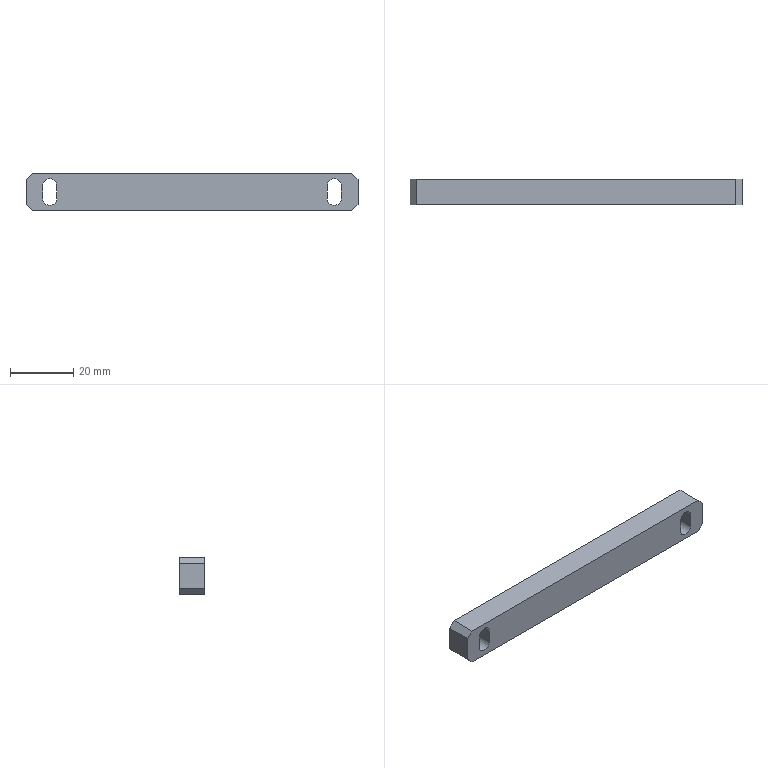Part | SolidWorks | features ICE 2, Chamfer 1, Extrusion 1 | 1 solid | 20 faces | box 105 x 8 x 12 mm | volume 9474 mm3 | plane 14 | cylinder 6 | commonest cylinder face diameters 4.5 x6
STEP:
#1=CARTESIAN_POINT('',(99.75,0.,-4.));
#2=VERTEX_POINT('',#1);
#3=CARTESIAN_POINT('',(97.5,0.,-1.75));
#4=VERTEX_POINT('',#3);
#5=CARTESIAN_POINT('',(97.5,0.,-4.));
#6=DIRECTION('',(0.,-1.,0.));
#7=DIRECTION('',(0.,0.,-1.));
#8=AXIS2_PLACEMENT_3D('',#5,#6,#7);
#9=CIRCLE('',#8,2.25);
#10=EDGE_CURVE('',#2,#4,#9,.T.);
#11=ORIENTED_EDGE('',*,*,#10,.T.);
#12=CARTESIAN_POINT('',(97.5,8.,-1.75));
#13=VERTEX_POINT('',#12);
#14=CARTESIAN_POINT('',(97.5,-2.,-1.75));
#15=DIRECTION('',(0.,1.,0.));
#16=VECTOR('',#15,1000.);
#17=LINE('',#14,#16);
#18=EDGE_CURVE('',#4,#13,#17,.T.);
#19=ORIENTED_EDGE('',*,*,#18,.T.);
#20=CARTESIAN_POINT('',(99.75,8.,-4.));
#21=VERTEX_POINT('',#20);
#22=CARTESIAN_POINT('',(97.5,8.,-4.));
#23=DIRECTION('',(0.,1.,0.));
#24=DIRECTION('',(0.,0.,-1.));
#25=AXIS2_PLACEMENT_3D('',#22,#23,#24);
#26=CIRCLE('',#25,2.25);
#27=EDGE_CURVE('',#13,#21,#26,.T.);
#28=ORIENTED_EDGE('',*,*,#27,.T.);
#29=CARTESIAN_POINT('',(99.75,-2.,-4.));
#30=DIRECTION('',(0.,1.,0.));
#31=VECTOR('',#30,1000.);
#32=LINE('',#29,#31);
#33=EDGE_CURVE('',#2,#21,#32,.T.);
#34=ORIENTED_EDGE('',*,*,#33,.F.);
#35=EDGE_LOOP('',(#11,#19,#28,#34));
#36=FACE_OUTER_BOUND('',#35,.T.);
#37=CARTESIAN_POINT('',(97.5,-2.,-4.));
#38=DIRECTION('',(0.,1.,0.));
#39=DIRECTION('',(0.,0.,1.));
#40=AXIS2_PLACEMENT_3D('',#37,#38,#39);
#41=CYLINDRICAL_SURFACE('',#40,2.25);
#42=ADVANCED_FACE('',(#36),#41,.F.);
#43=CARTESIAN_POINT('',(9.75,0.,-4.));
#44=VERTEX_POINT('',#43);
#45=CARTESIAN_POINT('',(7.5,0.,-1.75));
#46=VERTEX_POINT('',#45);
#47=CARTESIAN_POINT('',(7.5,0.,-4.));
#48=DIRECTION('',(0.,-1.,0.));
#49=DIRECTION('',(0.,0.,-1.));
#50=AXIS2_PLACEMENT_3D('',#47,#48,#49);
#51=CIRCLE('',#50,2.25);
#52=EDGE_CURVE('',#44,#46,#51,.T.);
#53=ORIENTED_EDGE('',*,*,#52,.T.);
#54=CARTESIAN_POINT('',(7.5,8.,-1.75));
#55=VERTEX_POINT('',#54);
#56=CARTESIAN_POINT('',(7.5,-2.,-1.75));
#57=DIRECTION('',(0.,1.,0.));
#58=VECTOR('',#57,1000.);
#59=LINE('',#56,#58);
#60=EDGE_CURVE('',#46,#55,#59,.T.);
#61=ORIENTED_EDGE('',*,*,#60,.T.);
#62=CARTESIAN_POINT('',(9.75,8.,-4.));
#63=VERTEX_POINT('',#62);
#64=CARTESIAN_POINT('',(7.5,8.,-4.));
#65=DIRECTION('',(0.,1.,0.));
#66=DIRECTION('',(0.,0.,1.));
#67=AXIS2_PLACEMENT_3D('',#64,#65,#66);
#68=CIRCLE('',#67,2.25);
#69=EDGE_CURVE('',#55,#63,#68,.T.);
#70=ORIENTED_EDGE('',*,*,#69,.T.);
#71=CARTESIAN_POINT('',(9.75,-2.,-4.));
#72=DIRECTION('',(0.,1.,0.));
#73=VECTOR('',#72,1000.);
#74=LINE('',#71,#73);
#75=EDGE_CURVE('',#44,#63,#74,.T.);
#76=ORIENTED_EDGE('',*,*,#75,.F.);
#77=EDGE_LOOP('',(#53,#61,#70,#76));
#78=FACE_OUTER_BOUND('',#77,.T.);
#79=CARTESIAN_POINT('',(7.5,-2.,-4.));
#80=DIRECTION('',(0.,1.,0.));
#81=DIRECTION('',(0.,0.,1.));
#82=AXIS2_PLACEMENT_3D('',#79,#80,#81);
#83=CYLINDRICAL_SURFACE('',#82,2.25);
#84=ADVANCED_FACE('',(#78),#83,.F.);
#85=CARTESIAN_POINT('',(0.,0.,-10.));
#86=VERTEX_POINT('',#85);
#87=CARTESIAN_POINT('',(0.,0.,-2.));
#88=VERTEX_POINT('',#87);
#89=CARTESIAN_POINT('',(0.,0.,0.));
#90=DIRECTION('',(0.,0.,1.));
#91=VECTOR('',#90,1000.);
#92=LINE('',#89,#91);
#93=EDGE_CURVE('',#86,#88,#92,.T.);
#94=ORIENTED_EDGE('',*,*,#93,.T.);
#95=CARTESIAN_POINT('',(0.,8.,-2.));
#96=VERTEX_POINT('',#95);
#97=CARTESIAN_POINT('',(0.,8.,-2.));
#98=DIRECTION('',(0.,1.,0.));
#99=VECTOR('',#98,1000.);
#100=LINE('',#97,#99);
#101=EDGE_CURVE('',#88,#96,#100,.T.);
#102=ORIENTED_EDGE('',*,*,#101,.T.);
#103=CARTESIAN_POINT('',(0.,8.,-10.));
#104=VERTEX_POINT('',#103);
#105=CARTESIAN_POINT('',(0.,8.,0.));
#106=DIRECTION('',(0.,0.,1.));
#107=VECTOR('',#106,1000.);
#108=LINE('',#105,#107);
#109=EDGE_CURVE('',#104,#96,#108,.T.);
#110=ORIENTED_EDGE('',*,*,#109,.F.);
#111=CARTESIAN_POINT('',(0.,8.,-10.));
#112=DIRECTION('',(0.,-1.,0.));
#113=VECTOR('',#112,1000.);
#114=LINE('',#111,#113);
#115=EDGE_CURVE('',#104,#86,#114,.T.);
#116=ORIENTED_EDGE('',*,*,#115,.T.);
#117=EDGE_LOOP('',(#94,#102,#110,#116));
#118=FACE_OUTER_BOUND('',#117,.T.);
#119=CARTESIAN_POINT('',(0.,8.,0.));
#120=DIRECTION('',(1.,0.,0.));
#121=DIRECTION('',(0.,0.,-1.));
#122=AXIS2_PLACEMENT_3D('',#119,#120,#121);
#123=PLANE('',#122);
#124=ADVANCED_FACE('',(#118),#123,.F.);
#125=CARTESIAN_POINT('',(2.,0.,0.));
#126=VERTEX_POINT('',#125);
#127=CARTESIAN_POINT('',(103.,0.,0.));
#128=VERTEX_POINT('',#127);
#129=CARTESIAN_POINT('',(0.,0.,0.));
#130=DIRECTION('',(1.,0.,0.));
#131=VECTOR('',#130,1000.);
#132=LINE('',#129,#131);
#133=EDGE_CURVE('',#126,#128,#132,.T.);
#134=ORIENTED_EDGE('',*,*,#133,.T.);
#135=CARTESIAN_POINT('',(103.,8.,0.));
#136=VERTEX_POINT('',#135);
#137=CARTESIAN_POINT('',(103.,8.,0.));
#138=DIRECTION('',(0.,1.,0.));
#139=VECTOR('',#138,1000.);
#140=LINE('',#137,#139);
#141=EDGE_CURVE('',#128,#136,#140,.T.);
#142=ORIENTED_EDGE('',*,*,#141,.T.);
#143=CARTESIAN_POINT('',(2.,8.,0.));
#144=VERTEX_POINT('',#143);
#145=CARTESIAN_POINT('',(0.,8.,0.));
#146=DIRECTION('',(1.,0.,0.));
#147=VECTOR('',#146,1000.);
#148=LINE('',#145,#147);
#149=EDGE_CURVE('',#144,#136,#148,.T.);
#150=ORIENTED_EDGE('',*,*,#149,.F.);
#151=CARTESIAN_POINT('',(2.,8.,0.));
#152=DIRECTION('',(0.,-1.,0.));
#153=VECTOR('',#152,1000.);
#154=LINE('',#151,#153);
#155=EDGE_CURVE('',#144,#126,#154,.T.);
#156=ORIENTED_EDGE('',*,*,#155,.T.);
#157=EDGE_LOOP('',(#134,#142,#150,#156));
#158=FACE_OUTER_BOUND('',#157,.T.);
#159=CARTESIAN_POINT('',(0.,8.,0.));
#160=DIRECTION('',(0.,0.,-1.));
#161=DIRECTION('',(-1.,0.,0.));
#162=AXIS2_PLACEMENT_3D('',#159,#160,#161);
#163=PLANE('',#162);
#164=ADVANCED_FACE('',(#158),#163,.F.);
#165=CARTESIAN_POINT('',(105.,8.,-2.));
#166=VERTEX_POINT('',#165);
#167=CARTESIAN_POINT('',(105.,8.,-10.));
#168=VERTEX_POINT('',#167);
#169=CARTESIAN_POINT('',(105.,8.,0.));
#170=DIRECTION('',(0.,0.,-1.));
#171=VECTOR('',#170,1000.);
#172=LINE('',#169,#171);
#173=EDGE_CURVE('',#166,#168,#172,.T.);
#174=ORIENTED_EDGE('',*,*,#173,.F.);
#175=CARTESIAN_POINT('',(105.,0.,-2.));
#176=VERTEX_POINT('',#175);
#177=CARTESIAN_POINT('',(105.,8.,-2.));
#178=DIRECTION('',(0.,-1.,0.));
#179=VECTOR('',#178,1000.);
#180=LINE('',#177,#179);
#181=EDGE_CURVE('',#166,#176,#180,.T.);
#182=ORIENTED_EDGE('',*,*,#181,.T.);
#183=CARTESIAN_POINT('',(105.,0.,-10.));
#184=VERTEX_POINT('',#183);
#185=CARTESIAN_POINT('',(105.,0.,0.));
#186=DIRECTION('',(0.,0.,-1.));
#187=VECTOR('',#186,1000.);
#188=LINE('',#185,#187);
#189=EDGE_CURVE('',#176,#184,#188,.T.);
#190=ORIENTED_EDGE('',*,*,#189,.T.);
#191=CARTESIAN_POINT('',(105.,8.,-10.));
#192=DIRECTION('',(0.,1.,0.));
#193=VECTOR('',#192,1000.);
#194=LINE('',#191,#193);
#195=EDGE_CURVE('',#184,#168,#194,.T.);
#196=ORIENTED_EDGE('',*,*,#195,.T.);
#197=EDGE_LOOP('',(#174,#182,#190,#196));
#198=FACE_OUTER_BOUND('',#197,.T.);
#199=CARTESIAN_POINT('',(105.,8.,0.));
#200=DIRECTION('',(-1.,0.,0.));
#201=DIRECTION('',(0.,0.,1.));
#202=AXIS2_PLACEMENT_3D('',#199,#200,#201);
#203=PLANE('',#202);
#204=ADVANCED_FACE('',(#198),#203,.F.);
#205=CARTESIAN_POINT('',(103.,8.,-12.));
#206=VERTEX_POINT('',#205);
#207=CARTESIAN_POINT('',(2.,8.,-12.));
#208=VERTEX_POINT('',#207);
#209=CARTESIAN_POINT('',(0.,8.,-12.));
#210=DIRECTION('',(-1.,0.,0.));
#211=VECTOR('',#210,1000.);
#212=LINE('',#209,#211);
#213=EDGE_CURVE('',#206,#208,#212,.T.);
#214=ORIENTED_EDGE('',*,*,#213,.F.);
#215=CARTESIAN_POINT('',(103.,0.,-12.));
#216=VERTEX_POINT('',#215);
#217=CARTESIAN_POINT('',(103.,8.,-12.));
#218=DIRECTION('',(0.,-1.,0.));
#219=VECTOR('',#218,1000.);
#220=LINE('',#217,#219);
#221=EDGE_CURVE('',#206,#216,#220,.T.);
#222=ORIENTED_EDGE('',*,*,#221,.T.);
#223=CARTESIAN_POINT('',(2.,0.,-12.));
#224=VERTEX_POINT('',#223);
#225=CARTESIAN_POINT('',(0.,0.,-12.));
#226=DIRECTION('',(-1.,0.,0.));
#227=VECTOR('',#226,1000.);
#228=LINE('',#225,#227);
#229=EDGE_CURVE('',#216,#224,#228,.T.);
#230=ORIENTED_EDGE('',*,*,#229,.T.);
#231=CARTESIAN_POINT('',(2.,8.,-12.));
#232=DIRECTION('',(0.,1.,0.));
#233=VECTOR('',#232,1000.);
#234=LINE('',#231,#233);
#235=EDGE_CURVE('',#224,#208,#234,.T.);
#236=ORIENTED_EDGE('',*,*,#235,.T.);
#237=EDGE_LOOP('',(#214,#222,#230,#236));
#238=FACE_OUTER_BOUND('',#237,.T.);
#239=CARTESIAN_POINT('',(0.,8.,-12.));
#240=DIRECTION('',(0.,0.,1.));
#241=DIRECTION('',(1.,0.,0.));
#242=AXIS2_PLACEMENT_3D('',#239,#240,#241);
#243=PLANE('',#242);
#244=ADVANCED_FACE('',(#238),#243,.F.);
#245=CARTESIAN_POINT('',(99.75,8.,-8.));
#246=VERTEX_POINT('',#245);
#247=CARTESIAN_POINT('',(99.75,8.,-4.));
#248=DIRECTION('',(0.,0.,-1.));
#249=VECTOR('',#248,1000.);
#250=LINE('',#247,#249);
#251=EDGE_CURVE('',#21,#246,#250,.T.);
#252=ORIENTED_EDGE('',*,*,#251,.F.);
#253=ORIENTED_EDGE('',*,*,#27,.F.);
#254=CARTESIAN_POINT('',(95.25,8.,-4.));
#255=VERTEX_POINT('',#254);
#256=CARTESIAN_POINT('',(97.5,8.,-4.));
#257=DIRECTION('',(0.,1.,0.));
#258=DIRECTION('',(0.,0.,-1.));
#259=AXIS2_PLACEMENT_3D('',#256,#257,#258);
#260=CIRCLE('',#259,2.25);
#261=EDGE_CURVE('',#255,#13,#260,.T.);
#262=ORIENTED_EDGE('',*,*,#261,.F.);
#263=CARTESIAN_POINT('',(95.25,8.,-8.));
#264=VERTEX_POINT('',#263);
#265=CARTESIAN_POINT('',(95.25,8.,-4.));
#266=DIRECTION('',(0.,0.,1.));
#267=VECTOR('',#266,1000.);
#268=LINE('',#265,#267);
#269=EDGE_CURVE('',#264,#255,#268,.T.);
#270=ORIENTED_EDGE('',*,*,#269,.F.);
#271=CARTESIAN_POINT('',(97.5,8.,-8.));
#272=DIRECTION('',(0.,1.,0.));
#273=DIRECTION('',(0.,0.,-1.));
#274=AXIS2_PLACEMENT_3D('',#271,#272,#273);
#275=CIRCLE('',#274,2.25);
#276=EDGE_CURVE('',#246,#264,#275,.T.);
#277=ORIENTED_EDGE('',*,*,#276,.F.);
#278=EDGE_LOOP('',(#252,#253,#262,#270,#277));
#279=FACE_BOUND('',#278,.T.);
#280=CARTESIAN_POINT('',(9.75,8.,-8.));
#281=VERTEX_POINT('',#280);
#282=CARTESIAN_POINT('',(9.75,8.,-4.));
#283=DIRECTION('',(0.,0.,-1.));
#284=VECTOR('',#283,1000.);
#285=LINE('',#282,#284);
#286=EDGE_CURVE('',#63,#281,#285,.T.);
#287=ORIENTED_EDGE('',*,*,#286,.F.);
#288=ORIENTED_EDGE('',*,*,#69,.F.);
#289=CARTESIAN_POINT('',(5.25,8.,-4.));
#290=VERTEX_POINT('',#289);
#291=CARTESIAN_POINT('',(7.5,8.,-4.));
#292=DIRECTION('',(0.,1.,0.));
#293=DIRECTION('',(0.,0.,1.));
#294=AXIS2_PLACEMENT_3D('',#291,#292,#293);
#295=CIRCLE('',#294,2.25);
#296=EDGE_CURVE('',#290,#55,#295,.T.);
#297=ORIENTED_EDGE('',*,*,#296,.F.);
#298=CARTESIAN_POINT('',(5.25,8.,-8.));
#299=VERTEX_POINT('',#298);
#300=CARTESIAN_POINT('',(5.25,8.,-4.));
#301=DIRECTION('',(0.,0.,1.));
#302=VECTOR('',#301,1000.);
#303=LINE('',#300,#302);
#304=EDGE_CURVE('',#299,#290,#303,.T.);
#305=ORIENTED_EDGE('',*,*,#304,.F.);
#306=CARTESIAN_POINT('',(7.5,8.,-8.));
#307=DIRECTION('',(0.,1.,0.));
#308=DIRECTION('',(0.,0.,1.));
#309=AXIS2_PLACEMENT_3D('',#306,#307,#308);
#310=CIRCLE('',#309,2.25);
#311=EDGE_CURVE('',#281,#299,#310,.T.);
#312=ORIENTED_EDGE('',*,*,#311,.F.);
#313=EDGE_LOOP('',(#287,#288,#297,#305,#312));
#314=FACE_BOUND('',#313,.T.);
#315=ORIENTED_EDGE('',*,*,#149,.T.);
#316=CARTESIAN_POINT('',(105.,8.,-2.));
#317=DIRECTION('',(0.7071,0.,-0.7071));
#318=VECTOR('',#317,1000.);
#319=LINE('',#316,#318);
#320=EDGE_CURVE('',#136,#166,#319,.T.);
#321=ORIENTED_EDGE('',*,*,#320,.T.);
#322=ORIENTED_EDGE('',*,*,#173,.T.);
#323=CARTESIAN_POINT('',(103.,8.,-12.));
#324=DIRECTION('',(-0.7071,0.,-0.7071));
#325=VECTOR('',#324,1000.);
#326=LINE('',#323,#325);
#327=EDGE_CURVE('',#168,#206,#326,.T.);
#328=ORIENTED_EDGE('',*,*,#327,.T.);
#329=ORIENTED_EDGE('',*,*,#213,.T.);
#330=CARTESIAN_POINT('',(0.,8.,-10.));
#331=DIRECTION('',(-0.7071,0.,0.7071));
#332=VECTOR('',#331,1000.);
#333=LINE('',#330,#332);
#334=EDGE_CURVE('',#208,#104,#333,.T.);
#335=ORIENTED_EDGE('',*,*,#334,.T.);
#336=ORIENTED_EDGE('',*,*,#109,.T.);
#337=CARTESIAN_POINT('',(2.,8.,0.));
#338=DIRECTION('',(0.7071,0.,0.7071));
#339=VECTOR('',#338,1000.);
#340=LINE('',#337,#339);
#341=EDGE_CURVE('',#96,#144,#340,.T.);
#342=ORIENTED_EDGE('',*,*,#341,.T.);
#343=EDGE_LOOP('',(#315,#321,#322,#328,#329,#335,#336,#342));
#344=FACE_OUTER_BOUND('',#343,.T.);
#345=CARTESIAN_POINT('',(0.,8.,0.));
#346=DIRECTION('',(0.,-1.,0.));
#347=DIRECTION('',(0.,0.,-1.));
#348=AXIS2_PLACEMENT_3D('',#345,#346,#347);
#349=PLANE('',#348);
#350=ADVANCED_FACE('',(#279,#314,#344),#349,.F.);
#351=ORIENTED_EDGE('',*,*,#10,.F.);
#352=CARTESIAN_POINT('',(99.75,0.,-8.));
#353=VERTEX_POINT('',#352);
#354=CARTESIAN_POINT('',(99.75,0.,0.));
#355=DIRECTION('',(0.,0.,1.));
#356=VECTOR('',#355,1000.);
#357=LINE('',#354,#356);
#358=EDGE_CURVE('',#353,#2,#357,.T.);
#359=ORIENTED_EDGE('',*,*,#358,.F.);
#360=CARTESIAN_POINT('',(95.25,0.,-8.));
#361=VERTEX_POINT('',#360);
#362=CARTESIAN_POINT('',(97.5,0.,-8.));
#363=DIRECTION('',(0.,-1.,0.));
#364=DIRECTION('',(0.,0.,-1.));
#365=AXIS2_PLACEMENT_3D('',#362,#363,#364);
#366=CIRCLE('',#365,2.25);
#367=EDGE_CURVE('',#361,#353,#366,.T.);
#368=ORIENTED_EDGE('',*,*,#367,.F.);
#369=CARTESIAN_POINT('',(95.25,0.,-4.));
#370=VERTEX_POINT('',#369);
#371=CARTESIAN_POINT('',(95.25,0.,0.));
#372=DIRECTION('',(0.,0.,-1.));
#373=VECTOR('',#372,1000.);
#374=LINE('',#371,#373);
#375=EDGE_CURVE('',#370,#361,#374,.T.);
#376=ORIENTED_EDGE('',*,*,#375,.F.);
#377=CARTESIAN_POINT('',(97.5,0.,-4.));
#378=DIRECTION('',(0.,-1.,0.));
#379=DIRECTION('',(0.,0.,-1.));
#380=AXIS2_PLACEMENT_3D('',#377,#378,#379);
#381=CIRCLE('',#380,2.25);
#382=EDGE_CURVE('',#4,#370,#381,.T.);
#383=ORIENTED_EDGE('',*,*,#382,.F.);
#384=EDGE_LOOP('',(#351,#359,#368,#376,#383));
#385=FACE_BOUND('',#384,.T.);
#386=ORIENTED_EDGE('',*,*,#52,.F.);
#387=CARTESIAN_POINT('',(9.75,0.,-8.));
#388=VERTEX_POINT('',#387);
#389=CARTESIAN_POINT('',(9.75,0.,0.));
#390=DIRECTION('',(0.,0.,1.));
#391=VECTOR('',#390,1000.);
#392=LINE('',#389,#391);
#393=EDGE_CURVE('',#388,#44,#392,.T.);
#394=ORIENTED_EDGE('',*,*,#393,.F.);
#395=CARTESIAN_POINT('',(5.25,0.,-8.));
#396=VERTEX_POINT('',#395);
#397=CARTESIAN_POINT('',(7.5,0.,-8.));
#398=DIRECTION('',(0.,-1.,0.));
#399=DIRECTION('',(0.,0.,-1.));
#400=AXIS2_PLACEMENT_3D('',#397,#398,#399);
#401=CIRCLE('',#400,2.25);
#402=EDGE_CURVE('',#396,#388,#401,.T.);
#403=ORIENTED_EDGE('',*,*,#402,.F.);
#404=CARTESIAN_POINT('',(5.25,0.,-4.));
#405=VERTEX_POINT('',#404);
#406=CARTESIAN_POINT('',(5.25,0.,0.));
#407=DIRECTION('',(0.,0.,-1.));
#408=VECTOR('',#407,1000.);
#409=LINE('',#406,#408);
#410=EDGE_CURVE('',#405,#396,#409,.T.);
#411=ORIENTED_EDGE('',*,*,#410,.F.);
#412=CARTESIAN_POINT('',(7.5,0.,-4.));
#413=DIRECTION('',(0.,-1.,0.));
#414=DIRECTION('',(0.,0.,-1.));
#415=AXIS2_PLACEMENT_3D('',#412,#413,#414);
#416=CIRCLE('',#415,2.25);
#417=EDGE_CURVE('',#46,#405,#416,.T.);
#418=ORIENTED_EDGE('',*,*,#417,.F.);
#419=EDGE_LOOP('',(#386,#394,#403,#411,#418));
#420=FACE_BOUND('',#419,.T.);
#421=ORIENTED_EDGE('',*,*,#189,.F.);
#422=CARTESIAN_POINT('',(51.5,0.,51.5));
#423=DIRECTION('',(-0.7071,0.,0.7071));
#424=VECTOR('',#423,1000.);
#425=LINE('',#422,#424);
#426=EDGE_CURVE('',#176,#128,#425,.T.);
#427=ORIENTED_EDGE('',*,*,#426,.T.);
#428=ORIENTED_EDGE('',*,*,#133,.F.);
#429=CARTESIAN_POINT('',(1.,0.,-1.));
#430=DIRECTION('',(-0.7071,0.,-0.7071));
#431=VECTOR('',#430,1000.);
#432=LINE('',#429,#431);
#433=EDGE_CURVE('',#126,#88,#432,.T.);
#434=ORIENTED_EDGE('',*,*,#433,.T.);
#435=ORIENTED_EDGE('',*,*,#93,.F.);
#436=CARTESIAN_POINT('',(-5.,0.,-5.));
#437=DIRECTION('',(0.7071,0.,-0.7071));
#438=VECTOR('',#437,1000.);
#439=LINE('',#436,#438);
#440=EDGE_CURVE('',#86,#224,#439,.T.);
#441=ORIENTED_EDGE('',*,*,#440,.T.);
#442=ORIENTED_EDGE('',*,*,#229,.F.);
#443=CARTESIAN_POINT('',(57.5,0.,-57.5));
#444=DIRECTION('',(0.7071,0.,0.7071));
#445=VECTOR('',#444,1000.);
#446=LINE('',#443,#445);
#447=EDGE_CURVE('',#216,#184,#446,.T.);
#448=ORIENTED_EDGE('',*,*,#447,.T.);
#449=EDGE_LOOP('',(#421,#427,#428,#434,#435,#441,#442,#448));
#450=FACE_OUTER_BOUND('',#449,.T.);
#451=CARTESIAN_POINT('',(0.,0.,0.));
#452=DIRECTION('',(0.,-1.,0.));
#453=DIRECTION('',(0.,0.,-1.));
#454=AXIS2_PLACEMENT_3D('',#451,#452,#453);
#455=PLANE('',#454);
#456=ADVANCED_FACE('',(#385,#420,#450),#455,.T.);
#457=ORIENTED_EDGE('',*,*,#320,.F.);
#458=ORIENTED_EDGE('',*,*,#141,.F.);
#459=ORIENTED_EDGE('',*,*,#426,.F.);
#460=ORIENTED_EDGE('',*,*,#181,.F.);
#461=EDGE_LOOP('',(#457,#458,#459,#460));
#462=FACE_OUTER_BOUND('',#461,.T.);
#463=CARTESIAN_POINT('',(105.,8.,-2.));
#464=DIRECTION('',(-0.7071,0.,-0.7071));
#465=DIRECTION('',(0.,-1.,0.));
#466=AXIS2_PLACEMENT_3D('',#463,#464,#465);
#467=PLANE('',#466);
#468=ADVANCED_FACE('',(#462),#467,.F.);
#469=ORIENTED_EDGE('',*,*,#327,.F.);
#470=ORIENTED_EDGE('',*,*,#195,.F.);
#471=ORIENTED_EDGE('',*,*,#447,.F.);
#472=ORIENTED_EDGE('',*,*,#221,.F.);
#473=EDGE_LOOP('',(#469,#470,#471,#472));
#474=FACE_OUTER_BOUND('',#473,.T.);
#475=CARTESIAN_POINT('',(103.,8.,-12.));
#476=DIRECTION('',(-0.7071,0.,0.7071));
#477=DIRECTION('',(0.,-1.,0.));
#478=AXIS2_PLACEMENT_3D('',#475,#476,#477);
#479=PLANE('',#478);
#480=ADVANCED_FACE('',(#474),#479,.F.);
#481=ORIENTED_EDGE('',*,*,#341,.F.);
#482=ORIENTED_EDGE('',*,*,#101,.F.);
#483=ORIENTED_EDGE('',*,*,#433,.F.);
#484=ORIENTED_EDGE('',*,*,#155,.F.);
#485=EDGE_LOOP('',(#481,#482,#483,#484));
#486=FACE_OUTER_BOUND('',#485,.T.);
#487=CARTESIAN_POINT('',(2.,8.,0.));
#488=DIRECTION('',(0.7071,0.,-0.7071));
#489=DIRECTION('',(0.,-1.,0.));
#490=AXIS2_PLACEMENT_3D('',#487,#488,#489);
#491=PLANE('',#490);
#492=ADVANCED_FACE('',(#486),#491,.F.);
#493=ORIENTED_EDGE('',*,*,#334,.F.);
#494=ORIENTED_EDGE('',*,*,#235,.F.);
#495=ORIENTED_EDGE('',*,*,#440,.F.);
#496=ORIENTED_EDGE('',*,*,#115,.F.);
#497=EDGE_LOOP('',(#493,#494,#495,#496));
#498=FACE_OUTER_BOUND('',#497,.T.);
#499=CARTESIAN_POINT('',(0.,8.,-10.));
#500=DIRECTION('',(0.7071,0.,0.7071));
#501=DIRECTION('',(0.,-1.,0.));
#502=AXIS2_PLACEMENT_3D('',#499,#500,#501);
#503=PLANE('',#502);
#504=ADVANCED_FACE('',(#498),#503,.F.);
#505=ORIENTED_EDGE('',*,*,#410,.T.);
#506=CARTESIAN_POINT('',(5.25,-2.,-8.));
#507=DIRECTION('',(0.,1.,0.));
#508=VECTOR('',#507,1000.);
#509=LINE('',#506,#508);
#510=EDGE_CURVE('',#396,#299,#509,.T.);
#511=ORIENTED_EDGE('',*,*,#510,.T.);
#512=ORIENTED_EDGE('',*,*,#304,.T.);
#513=CARTESIAN_POINT('',(5.25,-2.,-4.));
#514=DIRECTION('',(0.,1.,0.));
#515=VECTOR('',#514,1000.);
#516=LINE('',#513,#515);
#517=EDGE_CURVE('',#405,#290,#516,.T.);
#518=ORIENTED_EDGE('',*,*,#517,.F.);
#519=EDGE_LOOP('',(#505,#511,#512,#518));
#520=FACE_OUTER_BOUND('',#519,.T.);
#521=CARTESIAN_POINT('',(5.25,-2.,-4.));
#522=DIRECTION('',(-1.,0.,0.));
#523=DIRECTION('',(0.,0.,1.));
#524=AXIS2_PLACEMENT_3D('',#521,#522,#523);
#525=PLANE('',#524);
#526=ADVANCED_FACE('',(#520),#525,.F.);
#527=ORIENTED_EDGE('',*,*,#393,.T.);
#528=ORIENTED_EDGE('',*,*,#75,.T.);
#529=ORIENTED_EDGE('',*,*,#286,.T.);
#530=CARTESIAN_POINT('',(9.75,-2.,-8.));
#531=DIRECTION('',(0.,1.,0.));
#532=VECTOR('',#531,1000.);
#533=LINE('',#530,#532);
#534=EDGE_CURVE('',#388,#281,#533,.T.);
#535=ORIENTED_EDGE('',*,*,#534,.F.);
#536=EDGE_LOOP('',(#527,#528,#529,#535));
#537=FACE_OUTER_BOUND('',#536,.T.);
#538=CARTESIAN_POINT('',(9.75,-2.,-4.));
#539=DIRECTION('',(1.,0.,0.));
#540=DIRECTION('',(0.,0.,-1.));
#541=AXIS2_PLACEMENT_3D('',#538,#539,#540);
#542=PLANE('',#541);
#543=ADVANCED_FACE('',(#537),#542,.F.);
#544=ORIENTED_EDGE('',*,*,#60,.F.);
#545=ORIENTED_EDGE('',*,*,#417,.T.);
#546=ORIENTED_EDGE('',*,*,#517,.T.);
#547=ORIENTED_EDGE('',*,*,#296,.T.);
#548=EDGE_LOOP('',(#544,#545,#546,#547));
#549=FACE_OUTER_BOUND('',#548,.T.);
#550=CARTESIAN_POINT('',(7.5,-2.,-4.));
#551=DIRECTION('',(0.,1.,0.));
#552=DIRECTION('',(0.,0.,1.));
#553=AXIS2_PLACEMENT_3D('',#550,#551,#552);
#554=CYLINDRICAL_SURFACE('',#553,2.25);
#555=ADVANCED_FACE('',(#549),#554,.F.);
#556=ORIENTED_EDGE('',*,*,#402,.T.);
#557=ORIENTED_EDGE('',*,*,#534,.T.);
#558=ORIENTED_EDGE('',*,*,#311,.T.);
#559=ORIENTED_EDGE('',*,*,#510,.F.);
#560=EDGE_LOOP('',(#556,#557,#558,#559));
#561=FACE_OUTER_BOUND('',#560,.T.);
#562=CARTESIAN_POINT('',(7.5,-2.,-8.));
#563=DIRECTION('',(0.,1.,0.));
#564=DIRECTION('',(0.,0.,1.));
#565=AXIS2_PLACEMENT_3D('',#562,#563,#564);
#566=CYLINDRICAL_SURFACE('',#565,2.25);
#567=ADVANCED_FACE('',(#561),#566,.F.);
#568=ORIENTED_EDGE('',*,*,#375,.T.);
#569=CARTESIAN_POINT('',(95.25,-2.,-8.));
#570=DIRECTION('',(0.,1.,0.));
#571=VECTOR('',#570,1000.);
#572=LINE('',#569,#571);
#573=EDGE_CURVE('',#361,#264,#572,.T.);
#574=ORIENTED_EDGE('',*,*,#573,.T.);
#575=ORIENTED_EDGE('',*,*,#269,.T.);
#576=CARTESIAN_POINT('',(95.25,-2.,-4.));
#577=DIRECTION('',(0.,1.,0.));
#578=VECTOR('',#577,1000.);
#579=LINE('',#576,#578);
#580=EDGE_CURVE('',#370,#255,#579,.T.);
#581=ORIENTED_EDGE('',*,*,#580,.F.);
#582=EDGE_LOOP('',(#568,#574,#575,#581));
#583=FACE_OUTER_BOUND('',#582,.T.);
#584=CARTESIAN_POINT('',(95.25,-2.,-4.));
#585=DIRECTION('',(-1.,0.,0.));
#586=DIRECTION('',(0.,0.,1.));
#587=AXIS2_PLACEMENT_3D('',#584,#585,#586);
#588=PLANE('',#587);
#589=ADVANCED_FACE('',(#583),#588,.F.);
#590=ORIENTED_EDGE('',*,*,#358,.T.);
#591=ORIENTED_EDGE('',*,*,#33,.T.);
#592=ORIENTED_EDGE('',*,*,#251,.T.);
#593=CARTESIAN_POINT('',(99.75,-2.,-8.));
#594=DIRECTION('',(0.,1.,0.));
#595=VECTOR('',#594,1000.);
#596=LINE('',#593,#595);
#597=EDGE_CURVE('',#353,#246,#596,.T.);
#598=ORIENTED_EDGE('',*,*,#597,.F.);
#599=EDGE_LOOP('',(#590,#591,#592,#598));
#600=FACE_OUTER_BOUND('',#599,.T.);
#601=CARTESIAN_POINT('',(99.75,-2.,-4.));
#602=DIRECTION('',(1.,0.,0.));
#603=DIRECTION('',(0.,0.,-1.));
#604=AXIS2_PLACEMENT_3D('',#601,#602,#603);
#605=PLANE('',#604);
#606=ADVANCED_FACE('',(#600),#605,.F.);
#607=ORIENTED_EDGE('',*,*,#18,.F.);
#608=ORIENTED_EDGE('',*,*,#382,.T.);
#609=ORIENTED_EDGE('',*,*,#580,.T.);
#610=ORIENTED_EDGE('',*,*,#261,.T.);
#611=EDGE_LOOP('',(#607,#608,#609,#610));
#612=FACE_OUTER_BOUND('',#611,.T.);
#613=CARTESIAN_POINT('',(97.5,-2.,-4.));
#614=DIRECTION('',(0.,1.,0.));
#615=DIRECTION('',(0.,0.,1.));
#616=AXIS2_PLACEMENT_3D('',#613,#614,#615);
#617=CYLINDRICAL_SURFACE('',#616,2.25);
#618=ADVANCED_FACE('',(#612),#617,.F.);
#619=ORIENTED_EDGE('',*,*,#367,.T.);
#620=ORIENTED_EDGE('',*,*,#597,.T.);
#621=ORIENTED_EDGE('',*,*,#276,.T.);
#622=ORIENTED_EDGE('',*,*,#573,.F.);
#623=EDGE_LOOP('',(#619,#620,#621,#622));
#624=FACE_OUTER_BOUND('',#623,.T.);
#625=CARTESIAN_POINT('',(97.5,-2.,-8.));
#626=DIRECTION('',(0.,1.,0.));
#627=DIRECTION('',(0.,0.,1.));
#628=AXIS2_PLACEMENT_3D('',#625,#626,#627);
#629=CYLINDRICAL_SURFACE('',#628,2.25);
#630=ADVANCED_FACE('',(#624),#629,.F.);
#631=CLOSED_SHELL('',(#42,#84,#124,#164,#204,#244,#350,#456,#468,#480,#492,#504,#526,#543,#555,#567,#589,#606,#618,#630));
#632=MANIFOLD_SOLID_BREP('',#631);
#633=CARTESIAN_POINT('',(0.,0.,0.));
#634=DIRECTION('',(0.,0.,1.));
#635=DIRECTION('',(1.,0.,0.));
#636=AXIS2_PLACEMENT_3D('',#633,#634,#635);
#637=(LENGTH_UNIT()NAMED_UNIT(*)SI_UNIT(.MILLI.,.METRE.));
#638=UNCERTAINTY_MEASURE_WITH_UNIT(LENGTH_MEASURE(0.00001),#637,'','');
#639=(NAMED_UNIT(*)PLANE_ANGLE_UNIT()SI_UNIT($,.RADIAN.));
#640=(NAMED_UNIT(*)SI_UNIT($,.STERADIAN.)SOLID_ANGLE_UNIT());
#641=(GEOMETRIC_REPRESENTATION_CONTEXT(3)GLOBAL_UNCERTAINTY_ASSIGNED_CONTEXT((#638))GLOBAL_UNIT_ASSIGNED_CONTEXT((#637,#639,#640))REPRESENTATION_CONTEXT('',''));
#642=ADVANCED_BREP_SHAPE_REPRESENTATION('',(#632,#636),#641);